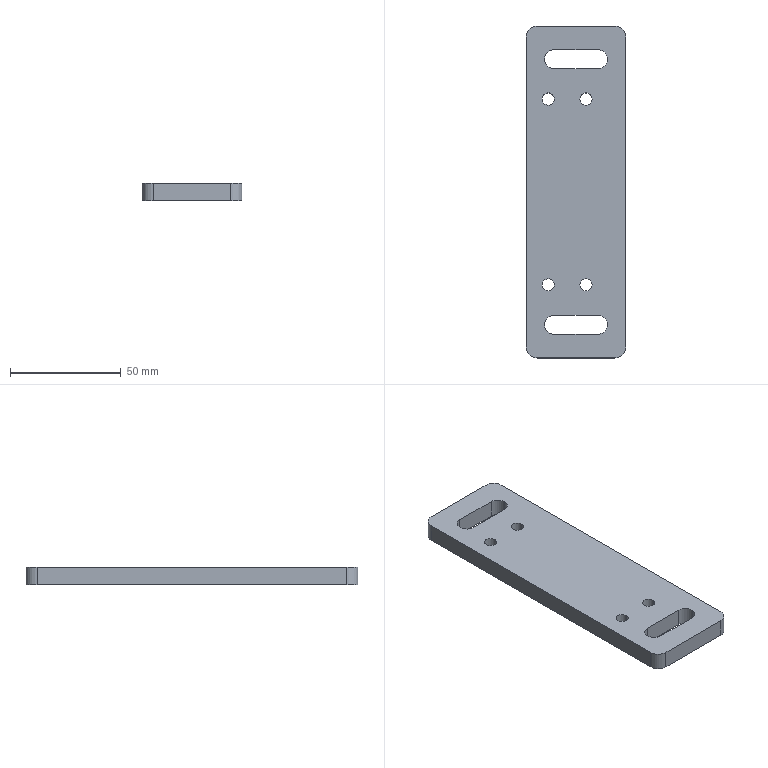Part | STEP file | 1 solid | 36 faces | box 45 x 150 x 8 mm | volume 48733 mm3 | cylinder 18 | plane 10 | cone 8 | commonest cylinder face diameters 5.5 x8 8.5 x6 10 x4